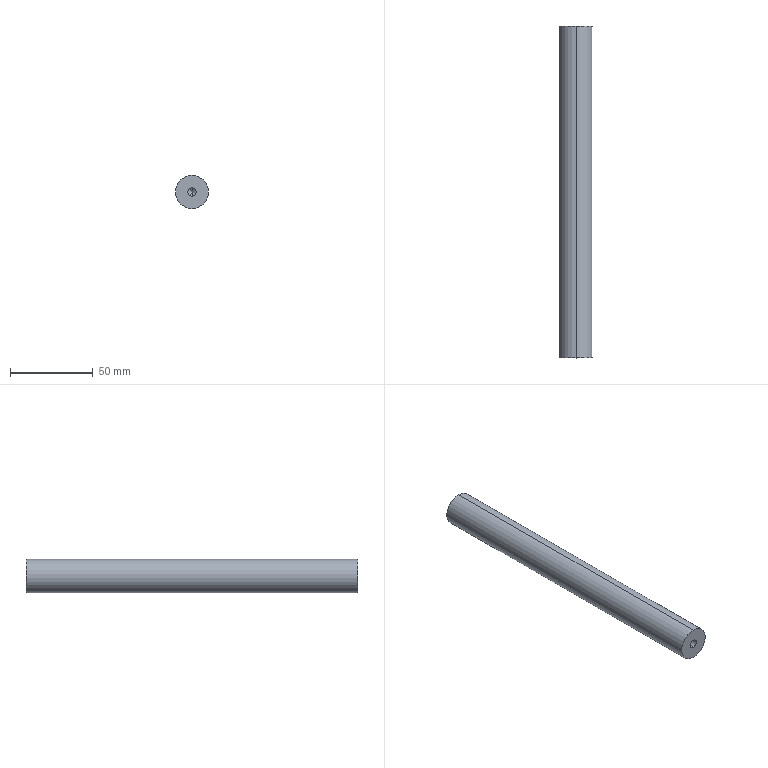Part | SolidWorks | features Extrusion 1, HoleWzd 1 | 1 solid | 8 faces | box 20 x 200 x 20 mm | volume 62527 mm3 | cylinder 4 | cone 2 | plane 2 | commonest cylinder face diameters 5 x2 20 x2
STEP:
#1=CARTESIAN_POINT('',(0.,15.,2.5));
#2=VERTEX_POINT('',#1);
#3=CARTESIAN_POINT('',(0.,15.,-2.5));
#4=VERTEX_POINT('',#3);
#5=CARTESIAN_POINT('',(0.,15.,0.));
#6=DIRECTION('',(0.,-1.,0.));
#7=DIRECTION('',(0.,0.,-1.));
#8=AXIS2_PLACEMENT_3D('',#5,#6,#7);
#9=CIRCLE('',#8,2.5);
#10=EDGE_CURVE('',#2,#4,#9,.T.);
#11=ORIENTED_EDGE('',*,*,#10,.F.);
#12=CARTESIAN_POINT('',(0.,0.,2.5));
#13=VERTEX_POINT('',#12);
#14=CARTESIAN_POINT('',(0.,0.,2.5));
#15=DIRECTION('',(0.,-1.,0.));
#16=VECTOR('',#15,1000.);
#17=LINE('',#14,#16);
#18=EDGE_CURVE('',#2,#13,#17,.T.);
#19=ORIENTED_EDGE('',*,*,#18,.T.);
#20=CARTESIAN_POINT('',(0.,0.,-2.5));
#21=VERTEX_POINT('',#20);
#22=CARTESIAN_POINT('',(0.,0.,0.));
#23=DIRECTION('',(0.,-1.,0.));
#24=DIRECTION('',(0.,0.,-1.));
#25=AXIS2_PLACEMENT_3D('',#22,#23,#24);
#26=CIRCLE('',#25,2.5);
#27=EDGE_CURVE('',#13,#21,#26,.T.);
#28=ORIENTED_EDGE('',*,*,#27,.T.);
#29=CARTESIAN_POINT('',(0.,0.,-2.5));
#30=DIRECTION('',(0.,-1.,0.));
#31=VECTOR('',#30,1000.);
#32=LINE('',#29,#31);
#33=EDGE_CURVE('',#4,#21,#32,.T.);
#34=ORIENTED_EDGE('',*,*,#33,.F.);
#35=EDGE_LOOP('',(#11,#19,#28,#34));
#36=FACE_OUTER_BOUND('',#35,.T.);
#37=CARTESIAN_POINT('',(0.,0.,0.));
#38=DIRECTION('',(0.,-1.,0.));
#39=DIRECTION('',(0.,0.,-1.));
#40=AXIS2_PLACEMENT_3D('',#37,#38,#39);
#41=CYLINDRICAL_SURFACE('',#40,2.5);
#42=ADVANCED_FACE('',(#36),#41,.F.);
#43=CARTESIAN_POINT('',(0.,16.502,0.));
#44=VERTEX_POINT('',#43);
#45=CARTESIAN_POINT('',(0.,15.,-2.5));
#46=DIRECTION('',(0.,-0.515,-0.8572));
#47=VECTOR('',#46,1000.);
#48=LINE('',#45,#47);
#49=EDGE_CURVE('',#44,#4,#48,.T.);
#50=ORIENTED_EDGE('',*,*,#49,.F.);
#51=CARTESIAN_POINT('',(0.,15.,2.5));
#52=DIRECTION('',(0.,-0.515,0.8572));
#53=VECTOR('',#52,1000.);
#54=LINE('',#51,#53);
#55=EDGE_CURVE('',#44,#2,#54,.T.);
#56=ORIENTED_EDGE('',*,*,#55,.T.);
#57=ORIENTED_EDGE('',*,*,#10,.T.);
#58=EDGE_LOOP('',(#50,#56,#57));
#59=FACE_OUTER_BOUND('',#58,.T.);
#60=CARTESIAN_POINT('',(0.,15.,0.));
#61=DIRECTION('',(0.,-1.,0.));
#62=DIRECTION('',(0.,0.,-1.));
#63=AXIS2_PLACEMENT_3D('',#60,#61,#62);
#64=CONICAL_SURFACE('',#63,2.5,1.03);
#65=ADVANCED_FACE('',(#59),#64,.F.);
#66=CARTESIAN_POINT('',(0.,200.,10.));
#67=VERTEX_POINT('',#66);
#68=CARTESIAN_POINT('',(0.,200.,-10.));
#69=VERTEX_POINT('',#68);
#70=CARTESIAN_POINT('',(0.,200.,0.));
#71=DIRECTION('',(0.,1.,0.));
#72=DIRECTION('',(0.,0.,1.));
#73=AXIS2_PLACEMENT_3D('',#70,#71,#72);
#74=CIRCLE('',#73,10.);
#75=EDGE_CURVE('',#67,#69,#74,.T.);
#76=ORIENTED_EDGE('',*,*,#75,.F.);
#77=CARTESIAN_POINT('',(0.,0.,10.));
#78=VERTEX_POINT('',#77);
#79=CARTESIAN_POINT('',(0.,200.,10.));
#80=DIRECTION('',(0.,-1.,0.));
#81=VECTOR('',#80,1000.);
#82=LINE('',#79,#81);
#83=EDGE_CURVE('',#67,#78,#82,.T.);
#84=ORIENTED_EDGE('',*,*,#83,.T.);
#85=CARTESIAN_POINT('',(0.,0.,-10.));
#86=VERTEX_POINT('',#85);
#87=CARTESIAN_POINT('',(0.,0.,0.));
#88=DIRECTION('',(0.,1.,0.));
#89=DIRECTION('',(0.,0.,1.));
#90=AXIS2_PLACEMENT_3D('',#87,#88,#89);
#91=CIRCLE('',#90,10.);
#92=EDGE_CURVE('',#78,#86,#91,.T.);
#93=ORIENTED_EDGE('',*,*,#92,.T.);
#94=CARTESIAN_POINT('',(0.,200.,-10.));
#95=DIRECTION('',(0.,-1.,0.));
#96=VECTOR('',#95,1000.);
#97=LINE('',#94,#96);
#98=EDGE_CURVE('',#69,#86,#97,.T.);
#99=ORIENTED_EDGE('',*,*,#98,.F.);
#100=EDGE_LOOP('',(#76,#84,#93,#99));
#101=FACE_OUTER_BOUND('',#100,.T.);
#102=CARTESIAN_POINT('',(0.,200.,0.));
#103=DIRECTION('',(0.,-1.,0.));
#104=DIRECTION('',(0.,0.,-1.));
#105=AXIS2_PLACEMENT_3D('',#102,#103,#104);
#106=CYLINDRICAL_SURFACE('',#105,10.);
#107=ADVANCED_FACE('',(#101),#106,.T.);
#108=ORIENTED_EDGE('',*,*,#83,.F.);
#109=CARTESIAN_POINT('',(0.,200.,0.));
#110=DIRECTION('',(0.,1.,0.));
#111=DIRECTION('',(0.,0.,1.));
#112=AXIS2_PLACEMENT_3D('',#109,#110,#111);
#113=CIRCLE('',#112,10.);
#114=EDGE_CURVE('',#69,#67,#113,.T.);
#115=ORIENTED_EDGE('',*,*,#114,.F.);
#116=ORIENTED_EDGE('',*,*,#98,.T.);
#117=CARTESIAN_POINT('',(0.,0.,0.));
#118=DIRECTION('',(0.,1.,0.));
#119=DIRECTION('',(0.,0.,1.));
#120=AXIS2_PLACEMENT_3D('',#117,#118,#119);
#121=CIRCLE('',#120,10.);
#122=EDGE_CURVE('',#86,#78,#121,.T.);
#123=ORIENTED_EDGE('',*,*,#122,.T.);
#124=EDGE_LOOP('',(#108,#115,#116,#123));
#125=FACE_OUTER_BOUND('',#124,.T.);
#126=CARTESIAN_POINT('',(0.,200.,0.));
#127=DIRECTION('',(0.,-1.,0.));
#128=DIRECTION('',(0.,0.,-1.));
#129=AXIS2_PLACEMENT_3D('',#126,#127,#128);
#130=CYLINDRICAL_SURFACE('',#129,10.);
#131=ADVANCED_FACE('',(#125),#130,.T.);
#132=ORIENTED_EDGE('',*,*,#114,.T.);
#133=ORIENTED_EDGE('',*,*,#75,.T.);
#134=EDGE_LOOP('',(#132,#133));
#135=FACE_OUTER_BOUND('',#134,.T.);
#136=CARTESIAN_POINT('',(0.,200.,0.));
#137=DIRECTION('',(0.,1.,0.));
#138=DIRECTION('',(0.,0.,1.));
#139=AXIS2_PLACEMENT_3D('',#136,#137,#138);
#140=PLANE('',#139);
#141=ADVANCED_FACE('',(#135),#140,.T.);
#142=CARTESIAN_POINT('',(0.,0.,0.));
#143=DIRECTION('',(0.,-1.,0.));
#144=DIRECTION('',(0.,0.,-1.));
#145=AXIS2_PLACEMENT_3D('',#142,#143,#144);
#146=CIRCLE('',#145,2.5);
#147=EDGE_CURVE('',#21,#13,#146,.T.);
#148=ORIENTED_EDGE('',*,*,#147,.F.);
#149=ORIENTED_EDGE('',*,*,#27,.F.);
#150=EDGE_LOOP('',(#148,#149));
#151=FACE_BOUND('',#150,.T.);
#152=ORIENTED_EDGE('',*,*,#122,.F.);
#153=ORIENTED_EDGE('',*,*,#92,.F.);
#154=EDGE_LOOP('',(#152,#153));
#155=FACE_OUTER_BOUND('',#154,.T.);
#156=CARTESIAN_POINT('',(0.,0.,0.));
#157=DIRECTION('',(0.,1.,0.));
#158=DIRECTION('',(0.,0.,1.));
#159=AXIS2_PLACEMENT_3D('',#156,#157,#158);
#160=PLANE('',#159);
#161=ADVANCED_FACE('',(#151,#155),#160,.F.);
#162=ORIENTED_EDGE('',*,*,#55,.F.);
#163=ORIENTED_EDGE('',*,*,#49,.T.);
#164=CARTESIAN_POINT('',(0.,15.,0.));
#165=DIRECTION('',(0.,-1.,0.));
#166=DIRECTION('',(0.,0.,-1.));
#167=AXIS2_PLACEMENT_3D('',#164,#165,#166);
#168=CIRCLE('',#167,2.5);
#169=EDGE_CURVE('',#4,#2,#168,.T.);
#170=ORIENTED_EDGE('',*,*,#169,.T.);
#171=EDGE_LOOP('',(#162,#163,#170));
#172=FACE_OUTER_BOUND('',#171,.T.);
#173=CARTESIAN_POINT('',(0.,15.,0.));
#174=DIRECTION('',(0.,-1.,0.));
#175=DIRECTION('',(0.,0.,-1.));
#176=AXIS2_PLACEMENT_3D('',#173,#174,#175);
#177=CONICAL_SURFACE('',#176,2.5,1.03);
#178=ADVANCED_FACE('',(#172),#177,.F.);
#179=ORIENTED_EDGE('',*,*,#18,.F.);
#180=ORIENTED_EDGE('',*,*,#169,.F.);
#181=ORIENTED_EDGE('',*,*,#33,.T.);
#182=ORIENTED_EDGE('',*,*,#147,.T.);
#183=EDGE_LOOP('',(#179,#180,#181,#182));
#184=FACE_OUTER_BOUND('',#183,.T.);
#185=CARTESIAN_POINT('',(0.,0.,0.));
#186=DIRECTION('',(0.,-1.,0.));
#187=DIRECTION('',(0.,0.,-1.));
#188=AXIS2_PLACEMENT_3D('',#185,#186,#187);
#189=CYLINDRICAL_SURFACE('',#188,2.5);
#190=ADVANCED_FACE('',(#184),#189,.F.);
#191=CLOSED_SHELL('',(#42,#65,#107,#131,#141,#161,#178,#190));
#192=MANIFOLD_SOLID_BREP('',#191);
#193=CARTESIAN_POINT('',(0.,0.,0.));
#194=DIRECTION('',(0.,0.,1.));
#195=DIRECTION('',(1.,0.,0.));
#196=AXIS2_PLACEMENT_3D('',#193,#194,#195);
#197=(LENGTH_UNIT()NAMED_UNIT(*)SI_UNIT(.MILLI.,.METRE.));
#198=UNCERTAINTY_MEASURE_WITH_UNIT(LENGTH_MEASURE(0.00001),#197,'','');
#199=(NAMED_UNIT(*)PLANE_ANGLE_UNIT()SI_UNIT($,.RADIAN.));
#200=(NAMED_UNIT(*)SI_UNIT($,.STERADIAN.)SOLID_ANGLE_UNIT());
#201=(GEOMETRIC_REPRESENTATION_CONTEXT(3)GLOBAL_UNCERTAINTY_ASSIGNED_CONTEXT((#198))GLOBAL_UNIT_ASSIGNED_CONTEXT((#197,#199,#200))REPRESENTATION_CONTEXT('',''));
#202=ADVANCED_BREP_SHAPE_REPRESENTATION('',(#192,#196),#201);